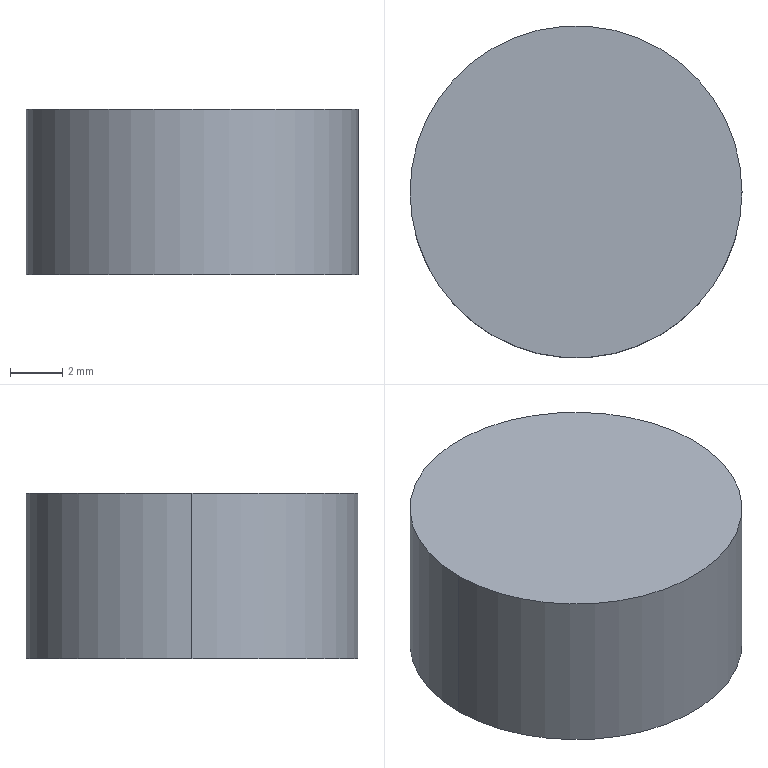Part | SolidWorks | features Extrusion 1 | 1 solid | 4 faces | box 12.7 x 12.7 x 6.35 mm | volume 804.398 mm3 | cylinder 2 | plane 2 | commonest cylinder face diameters 12.7 x2
STEP:
#1=CARTESIAN_POINT('',(6.35,0.,6.35));
#2=VERTEX_POINT('',#1);
#3=CARTESIAN_POINT('',(-6.35,0.,6.35));
#4=VERTEX_POINT('',#3);
#5=CARTESIAN_POINT('',(0.,0.,6.35));
#6=DIRECTION('',(0.,0.,1.));
#7=DIRECTION('',(1.,0.,0.));
#8=AXIS2_PLACEMENT_3D('',#5,#6,#7);
#9=CIRCLE('',#8,6.35);
#10=EDGE_CURVE('',#2,#4,#9,.T.);
#11=ORIENTED_EDGE('',*,*,#10,.F.);
#12=CARTESIAN_POINT('',(6.35,0.,0.));
#13=VERTEX_POINT('',#12);
#14=CARTESIAN_POINT('',(6.35,0.,6.35));
#15=DIRECTION('',(0.,0.,-1.));
#16=VECTOR('',#15,1000.);
#17=LINE('',#14,#16);
#18=EDGE_CURVE('',#2,#13,#17,.T.);
#19=ORIENTED_EDGE('',*,*,#18,.T.);
#20=CARTESIAN_POINT('',(-6.35,0.,0.));
#21=VERTEX_POINT('',#20);
#22=CARTESIAN_POINT('',(0.,0.,0.));
#23=DIRECTION('',(0.,0.,1.));
#24=DIRECTION('',(1.,0.,0.));
#25=AXIS2_PLACEMENT_3D('',#22,#23,#24);
#26=CIRCLE('',#25,6.35);
#27=EDGE_CURVE('',#13,#21,#26,.T.);
#28=ORIENTED_EDGE('',*,*,#27,.T.);
#29=CARTESIAN_POINT('',(-6.35,0.,6.35));
#30=DIRECTION('',(0.,0.,-1.));
#31=VECTOR('',#30,1000.);
#32=LINE('',#29,#31);
#33=EDGE_CURVE('',#4,#21,#32,.T.);
#34=ORIENTED_EDGE('',*,*,#33,.F.);
#35=EDGE_LOOP('',(#11,#19,#28,#34));
#36=FACE_OUTER_BOUND('',#35,.T.);
#37=CARTESIAN_POINT('',(0.,0.,6.35));
#38=DIRECTION('',(0.,0.,-1.));
#39=DIRECTION('',(-1.,0.,0.));
#40=AXIS2_PLACEMENT_3D('',#37,#38,#39);
#41=CYLINDRICAL_SURFACE('',#40,6.35);
#42=ADVANCED_FACE('',(#36),#41,.T.);
#43=ORIENTED_EDGE('',*,*,#18,.F.);
#44=CARTESIAN_POINT('',(0.,0.,6.35));
#45=DIRECTION('',(0.,0.,1.));
#46=DIRECTION('',(1.,0.,0.));
#47=AXIS2_PLACEMENT_3D('',#44,#45,#46);
#48=CIRCLE('',#47,6.35);
#49=EDGE_CURVE('',#4,#2,#48,.T.);
#50=ORIENTED_EDGE('',*,*,#49,.F.);
#51=ORIENTED_EDGE('',*,*,#33,.T.);
#52=CARTESIAN_POINT('',(0.,0.,0.));
#53=DIRECTION('',(0.,0.,1.));
#54=DIRECTION('',(1.,0.,0.));
#55=AXIS2_PLACEMENT_3D('',#52,#53,#54);
#56=CIRCLE('',#55,6.35);
#57=EDGE_CURVE('',#21,#13,#56,.T.);
#58=ORIENTED_EDGE('',*,*,#57,.T.);
#59=EDGE_LOOP('',(#43,#50,#51,#58));
#60=FACE_OUTER_BOUND('',#59,.T.);
#61=CARTESIAN_POINT('',(0.,0.,6.35));
#62=DIRECTION('',(0.,0.,-1.));
#63=DIRECTION('',(-1.,0.,0.));
#64=AXIS2_PLACEMENT_3D('',#61,#62,#63);
#65=CYLINDRICAL_SURFACE('',#64,6.35);
#66=ADVANCED_FACE('',(#60),#65,.T.);
#67=ORIENTED_EDGE('',*,*,#49,.T.);
#68=ORIENTED_EDGE('',*,*,#10,.T.);
#69=EDGE_LOOP('',(#67,#68));
#70=FACE_OUTER_BOUND('',#69,.T.);
#71=CARTESIAN_POINT('',(0.,0.,6.35));
#72=DIRECTION('',(0.,0.,1.));
#73=DIRECTION('',(1.,0.,0.));
#74=AXIS2_PLACEMENT_3D('',#71,#72,#73);
#75=PLANE('',#74);
#76=ADVANCED_FACE('',(#70),#75,.T.);
#77=ORIENTED_EDGE('',*,*,#57,.F.);
#78=ORIENTED_EDGE('',*,*,#27,.F.);
#79=EDGE_LOOP('',(#77,#78));
#80=FACE_OUTER_BOUND('',#79,.T.);
#81=CARTESIAN_POINT('',(0.,0.,0.));
#82=DIRECTION('',(0.,0.,1.));
#83=DIRECTION('',(1.,0.,0.));
#84=AXIS2_PLACEMENT_3D('',#81,#82,#83);
#85=PLANE('',#84);
#86=ADVANCED_FACE('',(#80),#85,.F.);
#87=CLOSED_SHELL('',(#42,#66,#76,#86));
#88=MANIFOLD_SOLID_BREP('',#87);
#89=CARTESIAN_POINT('',(0.,0.,0.));
#90=DIRECTION('',(0.,0.,1.));
#91=DIRECTION('',(1.,0.,0.));
#92=AXIS2_PLACEMENT_3D('',#89,#90,#91);
#93=(LENGTH_UNIT()NAMED_UNIT(*)SI_UNIT(.MILLI.,.METRE.));
#94=UNCERTAINTY_MEASURE_WITH_UNIT(LENGTH_MEASURE(0.00001),#93,'','');
#95=(NAMED_UNIT(*)PLANE_ANGLE_UNIT()SI_UNIT($,.RADIAN.));
#96=(NAMED_UNIT(*)SI_UNIT($,.STERADIAN.)SOLID_ANGLE_UNIT());
#97=(GEOMETRIC_REPRESENTATION_CONTEXT(3)GLOBAL_UNCERTAINTY_ASSIGNED_CONTEXT((#94))GLOBAL_UNIT_ASSIGNED_CONTEXT((#93,#95,#96))REPRESENTATION_CONTEXT('',''));
#98=ADVANCED_BREP_SHAPE_REPRESENTATION('',(#88,#92),#97);